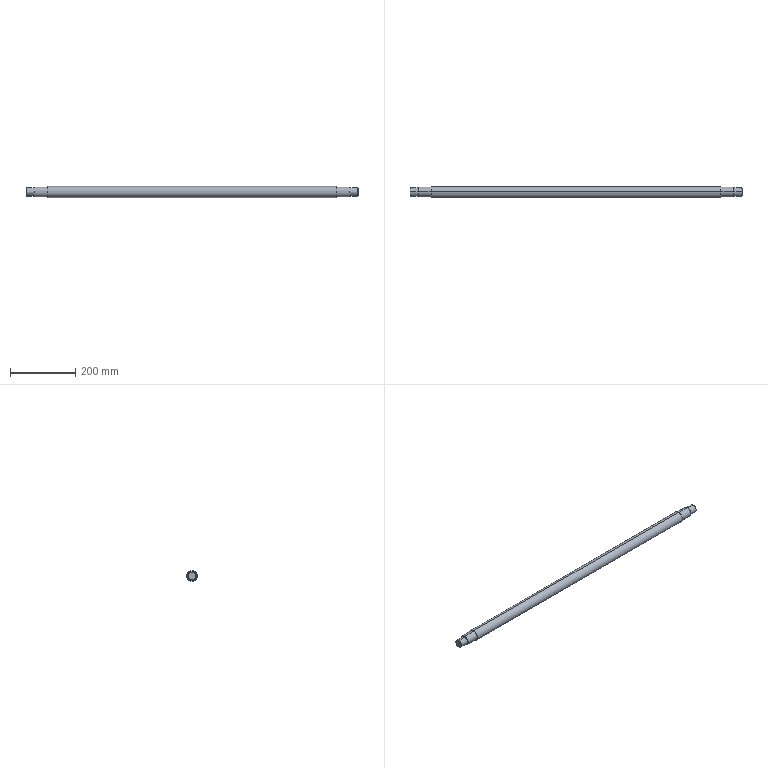Part | NX | features BREP 1 | 1 solid | 29 faces | box 1020 x 34 x 34 mm | volume 888390 mm3 | cylinder 12 | plane 9 | cone 8 | commonest cylinder face diameters 25 x4 30 x4 8 x2 34 x2
STEP:
#1=CARTESIAN_POINT('',(980.,0.,17.));
#2=VERTEX_POINT('',#1);
#3=CARTESIAN_POINT('',(980.,0.,-17.));
#4=VERTEX_POINT('',#3);
#5=CARTESIAN_POINT('',(980.,0.,0.));
#6=DIRECTION('',(-1.,0.,0.));
#7=DIRECTION('',(0.,0.,1.));
#8=AXIS2_PLACEMENT_3D('',#5,#6,#7);
#9=CIRCLE('',#8,17.);
#10=EDGE_CURVE('',#2,#4,#9,.T.);
#11=ORIENTED_EDGE('',*,*,#10,.T.);
#12=CARTESIAN_POINT('',(90.,0.,-17.));
#13=VERTEX_POINT('',#12);
#14=CARTESIAN_POINT('',(980.,0.,-17.));
#15=DIRECTION('',(-1.,0.,0.));
#16=VECTOR('',#15,1000.);
#17=LINE('',#14,#16);
#18=EDGE_CURVE('',#13,#4,#17,.F.);
#19=ORIENTED_EDGE('',*,*,#18,.F.);
#20=CARTESIAN_POINT('',(90.,0.,17.));
#21=VERTEX_POINT('',#20);
#22=CARTESIAN_POINT('',(90.,0.,0.));
#23=DIRECTION('',(1.,0.,0.));
#24=DIRECTION('',(0.,0.,1.));
#25=AXIS2_PLACEMENT_3D('',#22,#23,#24);
#26=CIRCLE('',#25,17.);
#27=EDGE_CURVE('',#13,#21,#26,.T.);
#28=ORIENTED_EDGE('',*,*,#27,.T.);
#29=CARTESIAN_POINT('',(980.,0.,17.));
#30=DIRECTION('',(-1.,0.,0.));
#31=VECTOR('',#30,1000.);
#32=LINE('',#29,#31);
#33=EDGE_CURVE('',#21,#2,#32,.F.);
#34=ORIENTED_EDGE('',*,*,#33,.T.);
#35=EDGE_LOOP('',(#11,#19,#28,#34));
#36=FACE_BOUND('',#35,.T.);
#37=CARTESIAN_POINT('',(980.,0.,0.));
#38=DIRECTION('',(-1.,0.,0.));
#39=DIRECTION('',(0.,0.,1.));
#40=AXIS2_PLACEMENT_3D('',#37,#38,#39);
#41=CYLINDRICAL_SURFACE('',#40,17.);
#42=ADVANCED_FACE('',(#36),#41,.T.);
#43=CARTESIAN_POINT('',(90.,0.,15.));
#44=VERTEX_POINT('',#43);
#45=CARTESIAN_POINT('',(90.,0.,-15.));
#46=VERTEX_POINT('',#45);
#47=CARTESIAN_POINT('',(90.,0.,0.));
#48=DIRECTION('',(-1.,0.,0.));
#49=DIRECTION('',(0.,0.,1.));
#50=AXIS2_PLACEMENT_3D('',#47,#48,#49);
#51=CIRCLE('',#50,15.);
#52=EDGE_CURVE('',#44,#46,#51,.T.);
#53=ORIENTED_EDGE('',*,*,#52,.T.);
#54=CARTESIAN_POINT('',(51.,0.,-15.));
#55=VERTEX_POINT('',#54);
#56=CARTESIAN_POINT('',(90.,0.,-15.));
#57=DIRECTION('',(-1.,0.,0.));
#58=VECTOR('',#57,1000.);
#59=LINE('',#56,#58);
#60=EDGE_CURVE('',#55,#46,#59,.F.);
#61=ORIENTED_EDGE('',*,*,#60,.F.);
#62=CARTESIAN_POINT('',(51.,0.,15.));
#63=VERTEX_POINT('',#62);
#64=CARTESIAN_POINT('',(51.,0.,0.));
#65=DIRECTION('',(1.,0.,0.));
#66=DIRECTION('',(0.,0.,1.));
#67=AXIS2_PLACEMENT_3D('',#64,#65,#66);
#68=CIRCLE('',#67,15.);
#69=EDGE_CURVE('',#55,#63,#68,.T.);
#70=ORIENTED_EDGE('',*,*,#69,.T.);
#71=CARTESIAN_POINT('',(90.,0.,15.));
#72=DIRECTION('',(-1.,0.,0.));
#73=VECTOR('',#72,1000.);
#74=LINE('',#71,#73);
#75=EDGE_CURVE('',#63,#44,#74,.F.);
#76=ORIENTED_EDGE('',*,*,#75,.T.);
#77=EDGE_LOOP('',(#53,#61,#70,#76));
#78=FACE_BOUND('',#77,.T.);
#79=CARTESIAN_POINT('',(81.,14.457,4.));
#80=VERTEX_POINT('',#79);
#81=CARTESIAN_POINT('',(64.,14.457,4.));
#82=VERTEX_POINT('',#81);
#83=CARTESIAN_POINT('',(90.,14.457,4.));
#84=DIRECTION('',(-1.,0.,0.));
#85=VECTOR('',#84,1000.);
#86=LINE('',#83,#85);
#87=EDGE_CURVE('',#80,#82,#86,.T.);
#88=ORIENTED_EDGE('',*,*,#87,.T.);
#89=CARTESIAN_POINT('',(64.,14.457,-4.));
#90=VERTEX_POINT('',#89);
#91=CARTESIAN_POINT('',(64.,14.457,4.));
#92=CARTESIAN_POINT('',(62.947,14.457,4.));
#93=CARTESIAN_POINT('',(60.87,14.733,3.133));
#94=CARTESIAN_POINT('',(59.565,15.133,0.005849));
#95=CARTESIAN_POINT('',(60.872,14.734,-3.134));
#96=CARTESIAN_POINT('',(62.938,14.457,-4.));
#97=CARTESIAN_POINT('',(64.,14.457,-4.));
#98=B_SPLINE_CURVE_WITH_KNOTS('',3,(#91,#92,#93,#94,#95,#96,#97),.UNSPECIFIED.,.F.,.F.,(4,1,1,1,4),(0.,0.25,0.5,0.75,1.),.UNSPECIFIED.);
#99=EDGE_CURVE('',#82,#90,#98,.T.);
#100=ORIENTED_EDGE('',*,*,#99,.T.);
#101=CARTESIAN_POINT('',(81.,14.457,-4.));
#102=VERTEX_POINT('',#101);
#103=CARTESIAN_POINT('',(90.,14.457,-4.));
#104=DIRECTION('',(1.,0.,0.));
#105=VECTOR('',#104,1000.);
#106=LINE('',#103,#105);
#107=EDGE_CURVE('',#90,#102,#106,.T.);
#108=ORIENTED_EDGE('',*,*,#107,.T.);
#109=CARTESIAN_POINT('',(81.,14.457,-4.));
#110=CARTESIAN_POINT('',(82.053,14.457,-4.));
#111=CARTESIAN_POINT('',(84.13,14.733,-3.133));
#112=CARTESIAN_POINT('',(85.435,15.133,-0.005849));
#113=CARTESIAN_POINT('',(84.128,14.734,3.134));
#114=CARTESIAN_POINT('',(82.062,14.457,4.));
#115=CARTESIAN_POINT('',(81.,14.457,4.));
#116=B_SPLINE_CURVE_WITH_KNOTS('',3,(#109,#110,#111,#112,#113,#114,#115),.UNSPECIFIED.,.F.,.F.,(4,1,1,1,4),(0.,0.25,0.5,0.75,1.),.UNSPECIFIED.);
#117=EDGE_CURVE('',#102,#80,#116,.T.);
#118=ORIENTED_EDGE('',*,*,#117,.T.);
#119=EDGE_LOOP('',(#88,#100,#108,#118));
#120=FACE_BOUND('',#119,.T.);
#121=CARTESIAN_POINT('',(90.,0.,0.));
#122=DIRECTION('',(-1.,0.,0.));
#123=DIRECTION('',(0.,0.,1.));
#124=AXIS2_PLACEMENT_3D('',#121,#122,#123);
#125=CYLINDRICAL_SURFACE('',#124,15.);
#126=ADVANCED_FACE('',(#78,#120),#125,.T.);
#127=CARTESIAN_POINT('',(1019.,0.,15.));
#128=VERTEX_POINT('',#127);
#129=CARTESIAN_POINT('',(1019.,0.,-15.));
#130=VERTEX_POINT('',#129);
#131=CARTESIAN_POINT('',(1019.,0.,0.));
#132=DIRECTION('',(-1.,0.,0.));
#133=DIRECTION('',(0.,0.,1.));
#134=AXIS2_PLACEMENT_3D('',#131,#132,#133);
#135=CIRCLE('',#134,15.);
#136=EDGE_CURVE('',#128,#130,#135,.T.);
#137=ORIENTED_EDGE('',*,*,#136,.T.);
#138=CARTESIAN_POINT('',(980.,0.,-15.));
#139=VERTEX_POINT('',#138);
#140=CARTESIAN_POINT('',(1020.,0.,-15.));
#141=DIRECTION('',(-1.,0.,0.));
#142=VECTOR('',#141,1000.);
#143=LINE('',#140,#142);
#144=EDGE_CURVE('',#139,#130,#143,.F.);
#145=ORIENTED_EDGE('',*,*,#144,.F.);
#146=CARTESIAN_POINT('',(980.,0.,15.));
#147=VERTEX_POINT('',#146);
#148=CARTESIAN_POINT('',(980.,0.,0.));
#149=DIRECTION('',(-1.,0.,0.));
#150=DIRECTION('',(0.,0.,1.));
#151=AXIS2_PLACEMENT_3D('',#148,#149,#150);
#152=CIRCLE('',#151,15.);
#153=EDGE_CURVE('',#147,#139,#152,.T.);
#154=ORIENTED_EDGE('',*,*,#153,.F.);
#155=CARTESIAN_POINT('',(1020.,0.,15.));
#156=DIRECTION('',(-1.,0.,0.));
#157=VECTOR('',#156,1000.);
#158=LINE('',#155,#157);
#159=EDGE_CURVE('',#147,#128,#158,.F.);
#160=ORIENTED_EDGE('',*,*,#159,.T.);
#161=EDGE_LOOP('',(#137,#145,#154,#160));
#162=FACE_BOUND('',#161,.T.);
#163=CARTESIAN_POINT('',(1020.,0.,0.));
#164=DIRECTION('',(-1.,0.,0.));
#165=DIRECTION('',(0.,0.,1.));
#166=AXIS2_PLACEMENT_3D('',#163,#164,#165);
#167=CYLINDRICAL_SURFACE('',#166,15.);
#168=ADVANCED_FACE('',(#162),#167,.T.);
#169=CARTESIAN_POINT('',(50.,0.,-14.));
#170=VERTEX_POINT('',#169);
#171=CARTESIAN_POINT('',(50.,0.,14.));
#172=VERTEX_POINT('',#171);
#173=CARTESIAN_POINT('',(50.,0.,0.));
#174=DIRECTION('',(1.,0.,0.));
#175=DIRECTION('',(0.,0.,-1.));
#176=AXIS2_PLACEMENT_3D('',#173,#174,#175);
#177=CIRCLE('',#176,14.);
#178=EDGE_CURVE('',#170,#172,#177,.T.);
#179=ORIENTED_EDGE('',*,*,#178,.T.);
#180=CARTESIAN_POINT('',(51.,0.,15.));
#181=DIRECTION('',(0.7071,0.,0.7071));
#182=VECTOR('',#181,1000.);
#183=LINE('',#180,#182);
#184=EDGE_CURVE('',#172,#63,#183,.T.);
#185=ORIENTED_EDGE('',*,*,#184,.T.);
#186=ORIENTED_EDGE('',*,*,#69,.F.);
#187=CARTESIAN_POINT('',(51.,0.,-15.));
#188=DIRECTION('',(0.7071,0.,-0.7071));
#189=VECTOR('',#188,1000.);
#190=LINE('',#187,#189);
#191=EDGE_CURVE('',#170,#55,#190,.T.);
#192=ORIENTED_EDGE('',*,*,#191,.F.);
#193=EDGE_LOOP('',(#179,#185,#186,#192));
#194=FACE_BOUND('',#193,.T.);
#195=CARTESIAN_POINT('',(51.,0.,0.));
#196=DIRECTION('',(1.,0.,0.));
#197=DIRECTION('',(0.,0.,-1.));
#198=AXIS2_PLACEMENT_3D('',#195,#196,#197);
#199=CONICAL_SURFACE('',#198,15.,0.7854);
#200=ADVANCED_FACE('',(#194),#199,.T.);
#201=CARTESIAN_POINT('',(1020.,0.,14.));
#202=VERTEX_POINT('',#201);
#203=CARTESIAN_POINT('',(1020.,0.,-14.));
#204=VERTEX_POINT('',#203);
#205=CARTESIAN_POINT('',(1020.,0.,0.));
#206=DIRECTION('',(-1.,0.,0.));
#207=DIRECTION('',(0.,0.,1.));
#208=AXIS2_PLACEMENT_3D('',#205,#206,#207);
#209=CIRCLE('',#208,14.);
#210=EDGE_CURVE('',#202,#204,#209,.T.);
#211=ORIENTED_EDGE('',*,*,#210,.T.);
#212=CARTESIAN_POINT('',(1019.,0.,-15.));
#213=DIRECTION('',(-0.7071,0.,-0.7071));
#214=VECTOR('',#213,1000.);
#215=LINE('',#212,#214);
#216=EDGE_CURVE('',#130,#204,#215,.F.);
#217=ORIENTED_EDGE('',*,*,#216,.F.);
#218=ORIENTED_EDGE('',*,*,#136,.F.);
#219=CARTESIAN_POINT('',(1019.,0.,15.));
#220=DIRECTION('',(-0.7071,0.,0.7071));
#221=VECTOR('',#220,1000.);
#222=LINE('',#219,#221);
#223=EDGE_CURVE('',#128,#202,#222,.F.);
#224=ORIENTED_EDGE('',*,*,#223,.T.);
#225=EDGE_LOOP('',(#211,#217,#218,#224));
#226=FACE_BOUND('',#225,.T.);
#227=CARTESIAN_POINT('',(1019.,0.,0.));
#228=DIRECTION('',(-1.,0.,0.));
#229=DIRECTION('',(0.,0.,1.));
#230=AXIS2_PLACEMENT_3D('',#227,#228,#229);
#231=CONICAL_SURFACE('',#230,15.,0.7854);
#232=ADVANCED_FACE('',(#226),#231,.T.);
#233=CARTESIAN_POINT('',(50.,0.,12.5));
#234=VERTEX_POINT('',#233);
#235=CARTESIAN_POINT('',(50.,0.,-12.5));
#236=VERTEX_POINT('',#235);
#237=CARTESIAN_POINT('',(50.,0.,0.));
#238=DIRECTION('',(-1.,0.,0.));
#239=DIRECTION('',(0.,0.,1.));
#240=AXIS2_PLACEMENT_3D('',#237,#238,#239);
#241=CIRCLE('',#240,12.5);
#242=EDGE_CURVE('',#234,#236,#241,.T.);
#243=ORIENTED_EDGE('',*,*,#242,.T.);
#244=CARTESIAN_POINT('',(26.,0.,-12.5));
#245=VERTEX_POINT('',#244);
#246=CARTESIAN_POINT('',(50.,0.,-12.5));
#247=DIRECTION('',(-1.,0.,0.));
#248=VECTOR('',#247,1000.);
#249=LINE('',#246,#248);
#250=EDGE_CURVE('',#245,#236,#249,.F.);
#251=ORIENTED_EDGE('',*,*,#250,.F.);
#252=CARTESIAN_POINT('',(26.,0.,12.5));
#253=VERTEX_POINT('',#252);
#254=CARTESIAN_POINT('',(26.,0.,0.));
#255=DIRECTION('',(1.,0.,0.));
#256=DIRECTION('',(0.,0.,1.));
#257=AXIS2_PLACEMENT_3D('',#254,#255,#256);
#258=CIRCLE('',#257,12.5);
#259=EDGE_CURVE('',#245,#253,#258,.T.);
#260=ORIENTED_EDGE('',*,*,#259,.T.);
#261=CARTESIAN_POINT('',(50.,0.,12.5));
#262=DIRECTION('',(-1.,0.,0.));
#263=VECTOR('',#262,1000.);
#264=LINE('',#261,#263);
#265=EDGE_CURVE('',#253,#234,#264,.F.);
#266=ORIENTED_EDGE('',*,*,#265,.T.);
#267=EDGE_LOOP('',(#243,#251,#260,#266));
#268=FACE_BOUND('',#267,.T.);
#269=CARTESIAN_POINT('',(50.,0.,0.));
#270=DIRECTION('',(-1.,0.,0.));
#271=DIRECTION('',(0.,0.,1.));
#272=AXIS2_PLACEMENT_3D('',#269,#270,#271);
#273=CYLINDRICAL_SURFACE('',#272,12.5);
#274=ADVANCED_FACE('',(#268),#273,.T.);
#275=CARTESIAN_POINT('',(1044.,0.,12.5));
#276=VERTEX_POINT('',#275);
#277=CARTESIAN_POINT('',(1044.,0.,-12.5));
#278=VERTEX_POINT('',#277);
#279=CARTESIAN_POINT('',(1044.,0.,0.));
#280=DIRECTION('',(-1.,0.,0.));
#281=DIRECTION('',(0.,0.,1.));
#282=AXIS2_PLACEMENT_3D('',#279,#280,#281);
#283=CIRCLE('',#282,12.5);
#284=EDGE_CURVE('',#276,#278,#283,.T.);
#285=ORIENTED_EDGE('',*,*,#284,.T.);
#286=CARTESIAN_POINT('',(1020.,0.,-12.5));
#287=VERTEX_POINT('',#286);
#288=CARTESIAN_POINT('',(1045.,0.,-12.5));
#289=DIRECTION('',(-1.,0.,0.));
#290=VECTOR('',#289,1000.);
#291=LINE('',#288,#290);
#292=EDGE_CURVE('',#287,#278,#291,.F.);
#293=ORIENTED_EDGE('',*,*,#292,.F.);
#294=CARTESIAN_POINT('',(1020.,0.,12.5));
#295=VERTEX_POINT('',#294);
#296=CARTESIAN_POINT('',(1020.,0.,0.));
#297=DIRECTION('',(-1.,0.,0.));
#298=DIRECTION('',(0.,0.,1.));
#299=AXIS2_PLACEMENT_3D('',#296,#297,#298);
#300=CIRCLE('',#299,12.5);
#301=EDGE_CURVE('',#295,#287,#300,.T.);
#302=ORIENTED_EDGE('',*,*,#301,.F.);
#303=CARTESIAN_POINT('',(1045.,0.,12.5));
#304=DIRECTION('',(-1.,0.,0.));
#305=VECTOR('',#304,1000.);
#306=LINE('',#303,#305);
#307=EDGE_CURVE('',#295,#276,#306,.F.);
#308=ORIENTED_EDGE('',*,*,#307,.T.);
#309=EDGE_LOOP('',(#285,#293,#302,#308));
#310=FACE_BOUND('',#309,.T.);
#311=CARTESIAN_POINT('',(1045.,0.,0.));
#312=DIRECTION('',(-1.,0.,0.));
#313=DIRECTION('',(0.,0.,1.));
#314=AXIS2_PLACEMENT_3D('',#311,#312,#313);
#315=CYLINDRICAL_SURFACE('',#314,12.5);
#316=ADVANCED_FACE('',(#310),#315,.T.);
#317=CARTESIAN_POINT('',(25.,0.,-11.5));
#318=VERTEX_POINT('',#317);
#319=CARTESIAN_POINT('',(25.,0.,11.5));
#320=VERTEX_POINT('',#319);
#321=CARTESIAN_POINT('',(25.,0.,0.));
#322=DIRECTION('',(1.,0.,0.));
#323=DIRECTION('',(0.,0.,-1.));
#324=AXIS2_PLACEMENT_3D('',#321,#322,#323);
#325=CIRCLE('',#324,11.5);
#326=EDGE_CURVE('',#318,#320,#325,.T.);
#327=ORIENTED_EDGE('',*,*,#326,.T.);
#328=CARTESIAN_POINT('',(26.,0.,12.5));
#329=DIRECTION('',(0.7071,0.,0.7071));
#330=VECTOR('',#329,1000.);
#331=LINE('',#328,#330);
#332=EDGE_CURVE('',#320,#253,#331,.T.);
#333=ORIENTED_EDGE('',*,*,#332,.T.);
#334=ORIENTED_EDGE('',*,*,#259,.F.);
#335=CARTESIAN_POINT('',(26.,0.,-12.5));
#336=DIRECTION('',(0.7071,0.,-0.7071));
#337=VECTOR('',#336,1000.);
#338=LINE('',#335,#337);
#339=EDGE_CURVE('',#318,#245,#338,.T.);
#340=ORIENTED_EDGE('',*,*,#339,.F.);
#341=EDGE_LOOP('',(#327,#333,#334,#340));
#342=FACE_BOUND('',#341,.T.);
#343=CARTESIAN_POINT('',(26.,0.,0.));
#344=DIRECTION('',(1.,0.,0.));
#345=DIRECTION('',(0.,0.,-1.));
#346=AXIS2_PLACEMENT_3D('',#343,#344,#345);
#347=CONICAL_SURFACE('',#346,12.5,0.7854);
#348=ADVANCED_FACE('',(#342),#347,.T.);
#349=CARTESIAN_POINT('',(1045.,0.,11.5));
#350=VERTEX_POINT('',#349);
#351=CARTESIAN_POINT('',(1045.,0.,-11.5));
#352=VERTEX_POINT('',#351);
#353=CARTESIAN_POINT('',(1045.,0.,0.));
#354=DIRECTION('',(-1.,0.,0.));
#355=DIRECTION('',(0.,0.,1.));
#356=AXIS2_PLACEMENT_3D('',#353,#354,#355);
#357=CIRCLE('',#356,11.5);
#358=EDGE_CURVE('',#350,#352,#357,.T.);
#359=ORIENTED_EDGE('',*,*,#358,.T.);
#360=CARTESIAN_POINT('',(1044.,0.,-12.5));
#361=DIRECTION('',(-0.7071,0.,-0.7071));
#362=VECTOR('',#361,1000.);
#363=LINE('',#360,#362);
#364=EDGE_CURVE('',#278,#352,#363,.F.);
#365=ORIENTED_EDGE('',*,*,#364,.F.);
#366=ORIENTED_EDGE('',*,*,#284,.F.);
#367=CARTESIAN_POINT('',(1044.,0.,12.5));
#368=DIRECTION('',(-0.7071,0.,0.7071));
#369=VECTOR('',#368,1000.);
#370=LINE('',#367,#369);
#371=EDGE_CURVE('',#276,#350,#370,.F.);
#372=ORIENTED_EDGE('',*,*,#371,.T.);
#373=EDGE_LOOP('',(#359,#365,#366,#372));
#374=FACE_BOUND('',#373,.T.);
#375=CARTESIAN_POINT('',(1044.,0.,0.));
#376=DIRECTION('',(-1.,0.,0.));
#377=DIRECTION('',(0.,0.,1.));
#378=AXIS2_PLACEMENT_3D('',#375,#376,#377);
#379=CONICAL_SURFACE('',#378,12.5,0.7854);
#380=ADVANCED_FACE('',(#374),#379,.T.);
#381=ORIENTED_EDGE('',*,*,#18,.T.);
#382=CARTESIAN_POINT('',(980.,0.,0.));
#383=DIRECTION('',(-1.,0.,0.));
#384=DIRECTION('',(0.,0.,1.));
#385=AXIS2_PLACEMENT_3D('',#382,#383,#384);
#386=CIRCLE('',#385,17.);
#387=EDGE_CURVE('',#4,#2,#386,.T.);
#388=ORIENTED_EDGE('',*,*,#387,.T.);
#389=ORIENTED_EDGE('',*,*,#33,.F.);
#390=CARTESIAN_POINT('',(90.,0.,0.));
#391=DIRECTION('',(1.,0.,0.));
#392=DIRECTION('',(0.,0.,1.));
#393=AXIS2_PLACEMENT_3D('',#390,#391,#392);
#394=CIRCLE('',#393,17.);
#395=EDGE_CURVE('',#21,#13,#394,.T.);
#396=ORIENTED_EDGE('',*,*,#395,.T.);
#397=EDGE_LOOP('',(#381,#388,#389,#396));
#398=FACE_BOUND('',#397,.T.);
#399=CARTESIAN_POINT('',(980.,0.,0.));
#400=DIRECTION('',(-1.,0.,0.));
#401=DIRECTION('',(0.,0.,1.));
#402=AXIS2_PLACEMENT_3D('',#399,#400,#401);
#403=CYLINDRICAL_SURFACE('',#402,17.);
#404=ADVANCED_FACE('',(#398),#403,.T.);
#405=ORIENTED_EDGE('',*,*,#395,.F.);
#406=ORIENTED_EDGE('',*,*,#27,.F.);
#407=EDGE_LOOP('',(#405,#406));
#408=FACE_BOUND('',#407,.T.);
#409=ORIENTED_EDGE('',*,*,#52,.F.);
#410=CARTESIAN_POINT('',(90.,0.,0.));
#411=DIRECTION('',(-1.,0.,0.));
#412=DIRECTION('',(0.,0.,1.));
#413=AXIS2_PLACEMENT_3D('',#410,#411,#412);
#414=CIRCLE('',#413,15.);
#415=EDGE_CURVE('',#46,#44,#414,.T.);
#416=ORIENTED_EDGE('',*,*,#415,.F.);
#417=EDGE_LOOP('',(#409,#416));
#418=FACE_BOUND('',#417,.T.);
#419=CARTESIAN_POINT('',(90.,0.,0.));
#420=DIRECTION('',(1.,0.,0.));
#421=DIRECTION('',(0.,1.,0.));
#422=AXIS2_PLACEMENT_3D('',#419,#420,#421);
#423=PLANE('',#422);
#424=ADVANCED_FACE('',(#408,#418),#423,.F.);
#425=ORIENTED_EDGE('',*,*,#10,.F.);
#426=ORIENTED_EDGE('',*,*,#387,.F.);
#427=EDGE_LOOP('',(#425,#426));
#428=FACE_BOUND('',#427,.T.);
#429=ORIENTED_EDGE('',*,*,#153,.T.);
#430=CARTESIAN_POINT('',(980.,0.,0.));
#431=DIRECTION('',(-1.,0.,0.));
#432=DIRECTION('',(0.,0.,1.));
#433=AXIS2_PLACEMENT_3D('',#430,#431,#432);
#434=CIRCLE('',#433,15.);
#435=EDGE_CURVE('',#139,#147,#434,.T.);
#436=ORIENTED_EDGE('',*,*,#435,.T.);
#437=EDGE_LOOP('',(#429,#436));
#438=FACE_BOUND('',#437,.T.);
#439=CARTESIAN_POINT('',(980.,0.,0.));
#440=DIRECTION('',(1.,0.,0.));
#441=DIRECTION('',(0.,1.,0.));
#442=AXIS2_PLACEMENT_3D('',#439,#440,#441);
#443=PLANE('',#442);
#444=ADVANCED_FACE('',(#428,#438),#443,.T.);
#445=ORIENTED_EDGE('',*,*,#60,.T.);
#446=ORIENTED_EDGE('',*,*,#415,.T.);
#447=ORIENTED_EDGE('',*,*,#75,.F.);
#448=CARTESIAN_POINT('',(51.,0.,0.));
#449=DIRECTION('',(1.,0.,0.));
#450=DIRECTION('',(0.,0.,1.));
#451=AXIS2_PLACEMENT_3D('',#448,#449,#450);
#452=CIRCLE('',#451,15.);
#453=EDGE_CURVE('',#63,#55,#452,.T.);
#454=ORIENTED_EDGE('',*,*,#453,.T.);
#455=EDGE_LOOP('',(#445,#446,#447,#454));
#456=FACE_BOUND('',#455,.T.);
#457=CARTESIAN_POINT('',(90.,0.,0.));
#458=DIRECTION('',(-1.,0.,0.));
#459=DIRECTION('',(0.,0.,1.));
#460=AXIS2_PLACEMENT_3D('',#457,#458,#459);
#461=CYLINDRICAL_SURFACE('',#460,15.);
#462=ADVANCED_FACE('',(#456),#461,.T.);
#463=ORIENTED_EDGE('',*,*,#144,.T.);
#464=CARTESIAN_POINT('',(1019.,0.,0.));
#465=DIRECTION('',(-1.,0.,0.));
#466=DIRECTION('',(0.,0.,1.));
#467=AXIS2_PLACEMENT_3D('',#464,#465,#466);
#468=CIRCLE('',#467,15.);
#469=EDGE_CURVE('',#130,#128,#468,.T.);
#470=ORIENTED_EDGE('',*,*,#469,.T.);
#471=ORIENTED_EDGE('',*,*,#159,.F.);
#472=ORIENTED_EDGE('',*,*,#435,.F.);
#473=EDGE_LOOP('',(#463,#470,#471,#472));
#474=FACE_BOUND('',#473,.T.);
#475=CARTESIAN_POINT('',(1020.,0.,0.));
#476=DIRECTION('',(-1.,0.,0.));
#477=DIRECTION('',(0.,0.,1.));
#478=AXIS2_PLACEMENT_3D('',#475,#476,#477);
#479=CYLINDRICAL_SURFACE('',#478,15.);
#480=ADVANCED_FACE('',(#474),#479,.T.);
#481=ORIENTED_EDGE('',*,*,#184,.F.);
#482=CARTESIAN_POINT('',(50.,0.,0.));
#483=DIRECTION('',(1.,0.,0.));
#484=DIRECTION('',(0.,0.,-1.));
#485=AXIS2_PLACEMENT_3D('',#482,#483,#484);
#486=CIRCLE('',#485,14.);
#487=EDGE_CURVE('',#172,#170,#486,.T.);
#488=ORIENTED_EDGE('',*,*,#487,.T.);
#489=ORIENTED_EDGE('',*,*,#191,.T.);
#490=ORIENTED_EDGE('',*,*,#453,.F.);
#491=EDGE_LOOP('',(#481,#488,#489,#490));
#492=FACE_BOUND('',#491,.T.);
#493=CARTESIAN_POINT('',(51.,0.,0.));
#494=DIRECTION('',(1.,0.,0.));
#495=DIRECTION('',(0.,0.,-1.));
#496=AXIS2_PLACEMENT_3D('',#493,#494,#495);
#497=CONICAL_SURFACE('',#496,15.,0.7854);
#498=ADVANCED_FACE('',(#492),#497,.T.);
#499=CARTESIAN_POINT('',(64.,11.7,-4.));
#500=VERTEX_POINT('',#499);
#501=CARTESIAN_POINT('',(64.,11.7,4.));
#502=VERTEX_POINT('',#501);
#503=CARTESIAN_POINT('',(64.,11.7,0.));
#504=DIRECTION('',(0.,1.,0.));
#505=DIRECTION('',(0.,0.,1.));
#506=AXIS2_PLACEMENT_3D('',#503,#504,#505);
#507=CIRCLE('',#506,4.);
#508=EDGE_CURVE('',#500,#502,#507,.T.);
#509=ORIENTED_EDGE('',*,*,#508,.F.);
#510=CARTESIAN_POINT('',(64.,11.7,-4.));
#511=DIRECTION('',(0.,-1.,0.));
#512=VECTOR('',#511,1000.);
#513=LINE('',#510,#512);
#514=EDGE_CURVE('',#90,#500,#513,.T.);
#515=ORIENTED_EDGE('',*,*,#514,.F.);
#516=ORIENTED_EDGE('',*,*,#99,.F.);
#517=CARTESIAN_POINT('',(64.,11.7,4.));
#518=DIRECTION('',(0.,1.,0.));
#519=VECTOR('',#518,1000.);
#520=LINE('',#517,#519);
#521=EDGE_CURVE('',#502,#82,#520,.T.);
#522=ORIENTED_EDGE('',*,*,#521,.F.);
#523=EDGE_LOOP('',(#509,#515,#516,#522));
#524=FACE_BOUND('',#523,.T.);
#525=CARTESIAN_POINT('',(64.,11.7,0.));
#526=DIRECTION('',(0.,1.,0.));
#527=DIRECTION('',(0.,0.,1.));
#528=AXIS2_PLACEMENT_3D('',#525,#526,#527);
#529=CYLINDRICAL_SURFACE('',#528,4.);
#530=ADVANCED_FACE('',(#524),#529,.F.);
#531=CARTESIAN_POINT('',(81.,11.7,4.));
#532=VERTEX_POINT('',#531);
#533=CARTESIAN_POINT('',(64.,11.7,4.));
#534=DIRECTION('',(1.,0.,0.));
#535=VECTOR('',#534,1000.);
#536=LINE('',#533,#535);
#537=EDGE_CURVE('',#502,#532,#536,.T.);
#538=ORIENTED_EDGE('',*,*,#537,.F.);
#539=ORIENTED_EDGE('',*,*,#521,.T.);
#540=ORIENTED_EDGE('',*,*,#87,.F.);
#541=CARTESIAN_POINT('',(81.,11.7,4.));
#542=DIRECTION('',(0.,1.,0.));
#543=VECTOR('',#542,1000.);
#544=LINE('',#541,#543);
#545=EDGE_CURVE('',#532,#80,#544,.T.);
#546=ORIENTED_EDGE('',*,*,#545,.F.);
#547=EDGE_LOOP('',(#538,#539,#540,#546));
#548=FACE_BOUND('',#547,.T.);
#549=CARTESIAN_POINT('',(64.,11.7,4.));
#550=DIRECTION('',(0.,0.,1.));
#551=DIRECTION('',(1.,0.,0.));
#552=AXIS2_PLACEMENT_3D('',#549,#550,#551);
#553=PLANE('',#552);
#554=ADVANCED_FACE('',(#548),#553,.F.);
#555=CARTESIAN_POINT('',(81.,11.7,-4.));
#556=VERTEX_POINT('',#555);
#557=CARTESIAN_POINT('',(81.,11.7,0.));
#558=DIRECTION('',(0.,1.,0.));
#559=DIRECTION('',(0.,0.,1.));
#560=AXIS2_PLACEMENT_3D('',#557,#558,#559);
#561=CIRCLE('',#560,4.);
#562=EDGE_CURVE('',#532,#556,#561,.T.);
#563=ORIENTED_EDGE('',*,*,#562,.F.);
#564=ORIENTED_EDGE('',*,*,#545,.T.);
#565=ORIENTED_EDGE('',*,*,#117,.F.);
#566=CARTESIAN_POINT('',(81.,11.7,-4.));
#567=DIRECTION('',(0.,1.,0.));
#568=VECTOR('',#567,1000.);
#569=LINE('',#566,#568);
#570=EDGE_CURVE('',#556,#102,#569,.T.);
#571=ORIENTED_EDGE('',*,*,#570,.F.);
#572=EDGE_LOOP('',(#563,#564,#565,#571));
#573=FACE_BOUND('',#572,.T.);
#574=CARTESIAN_POINT('',(81.,11.7,0.));
#575=DIRECTION('',(0.,1.,0.));
#576=DIRECTION('',(0.,0.,1.));
#577=AXIS2_PLACEMENT_3D('',#574,#575,#576);
#578=CYLINDRICAL_SURFACE('',#577,4.);
#579=ADVANCED_FACE('',(#573),#578,.F.);
#580=CARTESIAN_POINT('',(64.,11.7,-4.));
#581=DIRECTION('',(-1.,0.,0.));
#582=VECTOR('',#581,1000.);
#583=LINE('',#580,#582);
#584=EDGE_CURVE('',#556,#500,#583,.T.);
#585=ORIENTED_EDGE('',*,*,#584,.F.);
#586=ORIENTED_EDGE('',*,*,#570,.T.);
#587=ORIENTED_EDGE('',*,*,#107,.F.);
#588=ORIENTED_EDGE('',*,*,#514,.T.);
#589=EDGE_LOOP('',(#585,#586,#587,#588));
#590=FACE_BOUND('',#589,.T.);
#591=CARTESIAN_POINT('',(64.,11.7,-4.));
#592=DIRECTION('',(0.,0.,-1.));
#593=DIRECTION('',(0.,-1.,0.));
#594=AXIS2_PLACEMENT_3D('',#591,#592,#593);
#595=PLANE('',#594);
#596=ADVANCED_FACE('',(#590),#595,.F.);
#597=ORIENTED_EDGE('',*,*,#216,.T.);
#598=CARTESIAN_POINT('',(1020.,0.,0.));
#599=DIRECTION('',(-1.,0.,0.));
#600=DIRECTION('',(0.,0.,1.));
#601=AXIS2_PLACEMENT_3D('',#598,#599,#600);
#602=CIRCLE('',#601,14.);
#603=EDGE_CURVE('',#204,#202,#602,.T.);
#604=ORIENTED_EDGE('',*,*,#603,.T.);
#605=ORIENTED_EDGE('',*,*,#223,.F.);
#606=ORIENTED_EDGE('',*,*,#469,.F.);
#607=EDGE_LOOP('',(#597,#604,#605,#606));
#608=FACE_BOUND('',#607,.T.);
#609=CARTESIAN_POINT('',(1019.,0.,0.));
#610=DIRECTION('',(-1.,0.,0.));
#611=DIRECTION('',(0.,0.,1.));
#612=AXIS2_PLACEMENT_3D('',#609,#610,#611);
#613=CONICAL_SURFACE('',#612,15.,0.7854);
#614=ADVANCED_FACE('',(#608),#613,.T.);
#615=ORIENTED_EDGE('',*,*,#178,.F.);
#616=ORIENTED_EDGE('',*,*,#487,.F.);
#617=EDGE_LOOP('',(#615,#616));
#618=FACE_BOUND('',#617,.T.);
#619=ORIENTED_EDGE('',*,*,#242,.F.);
#620=CARTESIAN_POINT('',(50.,0.,0.));
#621=DIRECTION('',(-1.,0.,0.));
#622=DIRECTION('',(0.,0.,1.));
#623=AXIS2_PLACEMENT_3D('',#620,#621,#622);
#624=CIRCLE('',#623,12.5);
#625=EDGE_CURVE('',#236,#234,#624,.T.);
#626=ORIENTED_EDGE('',*,*,#625,.F.);
#627=EDGE_LOOP('',(#619,#626));
#628=FACE_BOUND('',#627,.T.);
#629=CARTESIAN_POINT('',(50.,0.,0.));
#630=DIRECTION('',(1.,0.,0.));
#631=DIRECTION('',(0.,1.,0.));
#632=AXIS2_PLACEMENT_3D('',#629,#630,#631);
#633=PLANE('',#632);
#634=ADVANCED_FACE('',(#618,#628),#633,.F.);
#635=ORIENTED_EDGE('',*,*,#537,.T.);
#636=ORIENTED_EDGE('',*,*,#562,.T.);
#637=ORIENTED_EDGE('',*,*,#584,.T.);
#638=ORIENTED_EDGE('',*,*,#508,.T.);
#639=EDGE_LOOP('',(#635,#636,#637,#638));
#640=FACE_BOUND('',#639,.T.);
#641=CARTESIAN_POINT('',(64.,11.7,0.));
#642=DIRECTION('',(0.,-1.,0.));
#643=DIRECTION('',(0.,0.,-1.));
#644=AXIS2_PLACEMENT_3D('',#641,#642,#643);
#645=PLANE('',#644);
#646=ADVANCED_FACE('',(#640),#645,.F.);
#647=ORIENTED_EDGE('',*,*,#210,.F.);
#648=ORIENTED_EDGE('',*,*,#603,.F.);
#649=EDGE_LOOP('',(#647,#648));
#650=FACE_BOUND('',#649,.T.);
#651=ORIENTED_EDGE('',*,*,#301,.T.);
#652=CARTESIAN_POINT('',(1020.,0.,0.));
#653=DIRECTION('',(-1.,0.,0.));
#654=DIRECTION('',(0.,0.,1.));
#655=AXIS2_PLACEMENT_3D('',#652,#653,#654);
#656=CIRCLE('',#655,12.5);
#657=EDGE_CURVE('',#287,#295,#656,.T.);
#658=ORIENTED_EDGE('',*,*,#657,.T.);
#659=EDGE_LOOP('',(#651,#658));
#660=FACE_BOUND('',#659,.T.);
#661=CARTESIAN_POINT('',(1020.,0.,0.));
#662=DIRECTION('',(1.,0.,0.));
#663=DIRECTION('',(0.,1.,0.));
#664=AXIS2_PLACEMENT_3D('',#661,#662,#663);
#665=PLANE('',#664);
#666=ADVANCED_FACE('',(#650,#660),#665,.T.);
#667=ORIENTED_EDGE('',*,*,#250,.T.);
#668=ORIENTED_EDGE('',*,*,#625,.T.);
#669=ORIENTED_EDGE('',*,*,#265,.F.);
#670=CARTESIAN_POINT('',(26.,0.,0.));
#671=DIRECTION('',(1.,0.,0.));
#672=DIRECTION('',(0.,0.,1.));
#673=AXIS2_PLACEMENT_3D('',#670,#671,#672);
#674=CIRCLE('',#673,12.5);
#675=EDGE_CURVE('',#253,#245,#674,.T.);
#676=ORIENTED_EDGE('',*,*,#675,.T.);
#677=EDGE_LOOP('',(#667,#668,#669,#676));
#678=FACE_BOUND('',#677,.T.);
#679=CARTESIAN_POINT('',(50.,0.,0.));
#680=DIRECTION('',(-1.,0.,0.));
#681=DIRECTION('',(0.,0.,1.));
#682=AXIS2_PLACEMENT_3D('',#679,#680,#681);
#683=CYLINDRICAL_SURFACE('',#682,12.5);
#684=ADVANCED_FACE('',(#678),#683,.T.);
#685=ORIENTED_EDGE('',*,*,#292,.T.);
#686=CARTESIAN_POINT('',(1044.,0.,0.));
#687=DIRECTION('',(-1.,0.,0.));
#688=DIRECTION('',(0.,0.,1.));
#689=AXIS2_PLACEMENT_3D('',#686,#687,#688);
#690=CIRCLE('',#689,12.5);
#691=EDGE_CURVE('',#278,#276,#690,.T.);
#692=ORIENTED_EDGE('',*,*,#691,.T.);
#693=ORIENTED_EDGE('',*,*,#307,.F.);
#694=ORIENTED_EDGE('',*,*,#657,.F.);
#695=EDGE_LOOP('',(#685,#692,#693,#694));
#696=FACE_BOUND('',#695,.T.);
#697=CARTESIAN_POINT('',(1045.,0.,0.));
#698=DIRECTION('',(-1.,0.,0.));
#699=DIRECTION('',(0.,0.,1.));
#700=AXIS2_PLACEMENT_3D('',#697,#698,#699);
#701=CYLINDRICAL_SURFACE('',#700,12.5);
#702=ADVANCED_FACE('',(#696),#701,.T.);
#703=ORIENTED_EDGE('',*,*,#332,.F.);
#704=CARTESIAN_POINT('',(25.,0.,0.));
#705=DIRECTION('',(1.,0.,0.));
#706=DIRECTION('',(0.,0.,-1.));
#707=AXIS2_PLACEMENT_3D('',#704,#705,#706);
#708=CIRCLE('',#707,11.5);
#709=EDGE_CURVE('',#320,#318,#708,.T.);
#710=ORIENTED_EDGE('',*,*,#709,.T.);
#711=ORIENTED_EDGE('',*,*,#339,.T.);
#712=ORIENTED_EDGE('',*,*,#675,.F.);
#713=EDGE_LOOP('',(#703,#710,#711,#712));
#714=FACE_BOUND('',#713,.T.);
#715=CARTESIAN_POINT('',(26.,0.,0.));
#716=DIRECTION('',(1.,0.,0.));
#717=DIRECTION('',(0.,0.,-1.));
#718=AXIS2_PLACEMENT_3D('',#715,#716,#717);
#719=CONICAL_SURFACE('',#718,12.5,0.7854);
#720=ADVANCED_FACE('',(#714),#719,.T.);
#721=ORIENTED_EDGE('',*,*,#364,.T.);
#722=CARTESIAN_POINT('',(1045.,0.,0.));
#723=DIRECTION('',(-1.,0.,0.));
#724=DIRECTION('',(0.,0.,1.));
#725=AXIS2_PLACEMENT_3D('',#722,#723,#724);
#726=CIRCLE('',#725,11.5);
#727=EDGE_CURVE('',#352,#350,#726,.T.);
#728=ORIENTED_EDGE('',*,*,#727,.T.);
#729=ORIENTED_EDGE('',*,*,#371,.F.);
#730=ORIENTED_EDGE('',*,*,#691,.F.);
#731=EDGE_LOOP('',(#721,#728,#729,#730));
#732=FACE_BOUND('',#731,.T.);
#733=CARTESIAN_POINT('',(1044.,0.,0.));
#734=DIRECTION('',(-1.,0.,0.));
#735=DIRECTION('',(0.,0.,1.));
#736=AXIS2_PLACEMENT_3D('',#733,#734,#735);
#737=CONICAL_SURFACE('',#736,12.5,0.7854);
#738=ADVANCED_FACE('',(#732),#737,.T.);
#739=ORIENTED_EDGE('',*,*,#326,.F.);
#740=ORIENTED_EDGE('',*,*,#709,.F.);
#741=EDGE_LOOP('',(#739,#740));
#742=FACE_BOUND('',#741,.T.);
#743=CARTESIAN_POINT('',(25.,0.,0.));
#744=DIRECTION('',(1.,0.,0.));
#745=DIRECTION('',(0.,1.,0.));
#746=AXIS2_PLACEMENT_3D('',#743,#744,#745);
#747=PLANE('',#746);
#748=ADVANCED_FACE('',(#742),#747,.F.);
#749=ORIENTED_EDGE('',*,*,#358,.F.);
#750=ORIENTED_EDGE('',*,*,#727,.F.);
#751=EDGE_LOOP('',(#749,#750));
#752=FACE_BOUND('',#751,.T.);
#753=CARTESIAN_POINT('',(1045.,0.,0.));
#754=DIRECTION('',(1.,0.,0.));
#755=DIRECTION('',(0.,1.,0.));
#756=AXIS2_PLACEMENT_3D('',#753,#754,#755);
#757=PLANE('',#756);
#758=ADVANCED_FACE('',(#752),#757,.T.);
#759=CLOSED_SHELL('',(#42,#126,#168,#200,#232,#274,#316,#348,#380,#404,#424,#444,#462,#480,#498,#530,#554,#579,#596,#614,#634,#646,#666,#684,#702,#720,#738,#748,#758));
#760=MANIFOLD_SOLID_BREP('',#759);
#761=(LENGTH_UNIT()NAMED_UNIT(*)SI_UNIT(.MILLI.,.METRE.));
#762=UNCERTAINTY_MEASURE_WITH_UNIT(LENGTH_MEASURE(0.0508),#761,'','');
#763=(NAMED_UNIT(*)PLANE_ANGLE_UNIT()SI_UNIT($,.RADIAN.));
#764=(NAMED_UNIT(*)SI_UNIT($,.STERADIAN.)SOLID_ANGLE_UNIT());
#765=(GEOMETRIC_REPRESENTATION_CONTEXT(3)GLOBAL_UNCERTAINTY_ASSIGNED_CONTEXT((#762))GLOBAL_UNIT_ASSIGNED_CONTEXT((#761,#763,#764))REPRESENTATION_CONTEXT('',''));
#766=ADVANCED_BREP_SHAPE_REPRESENTATION('',(#760),#765);